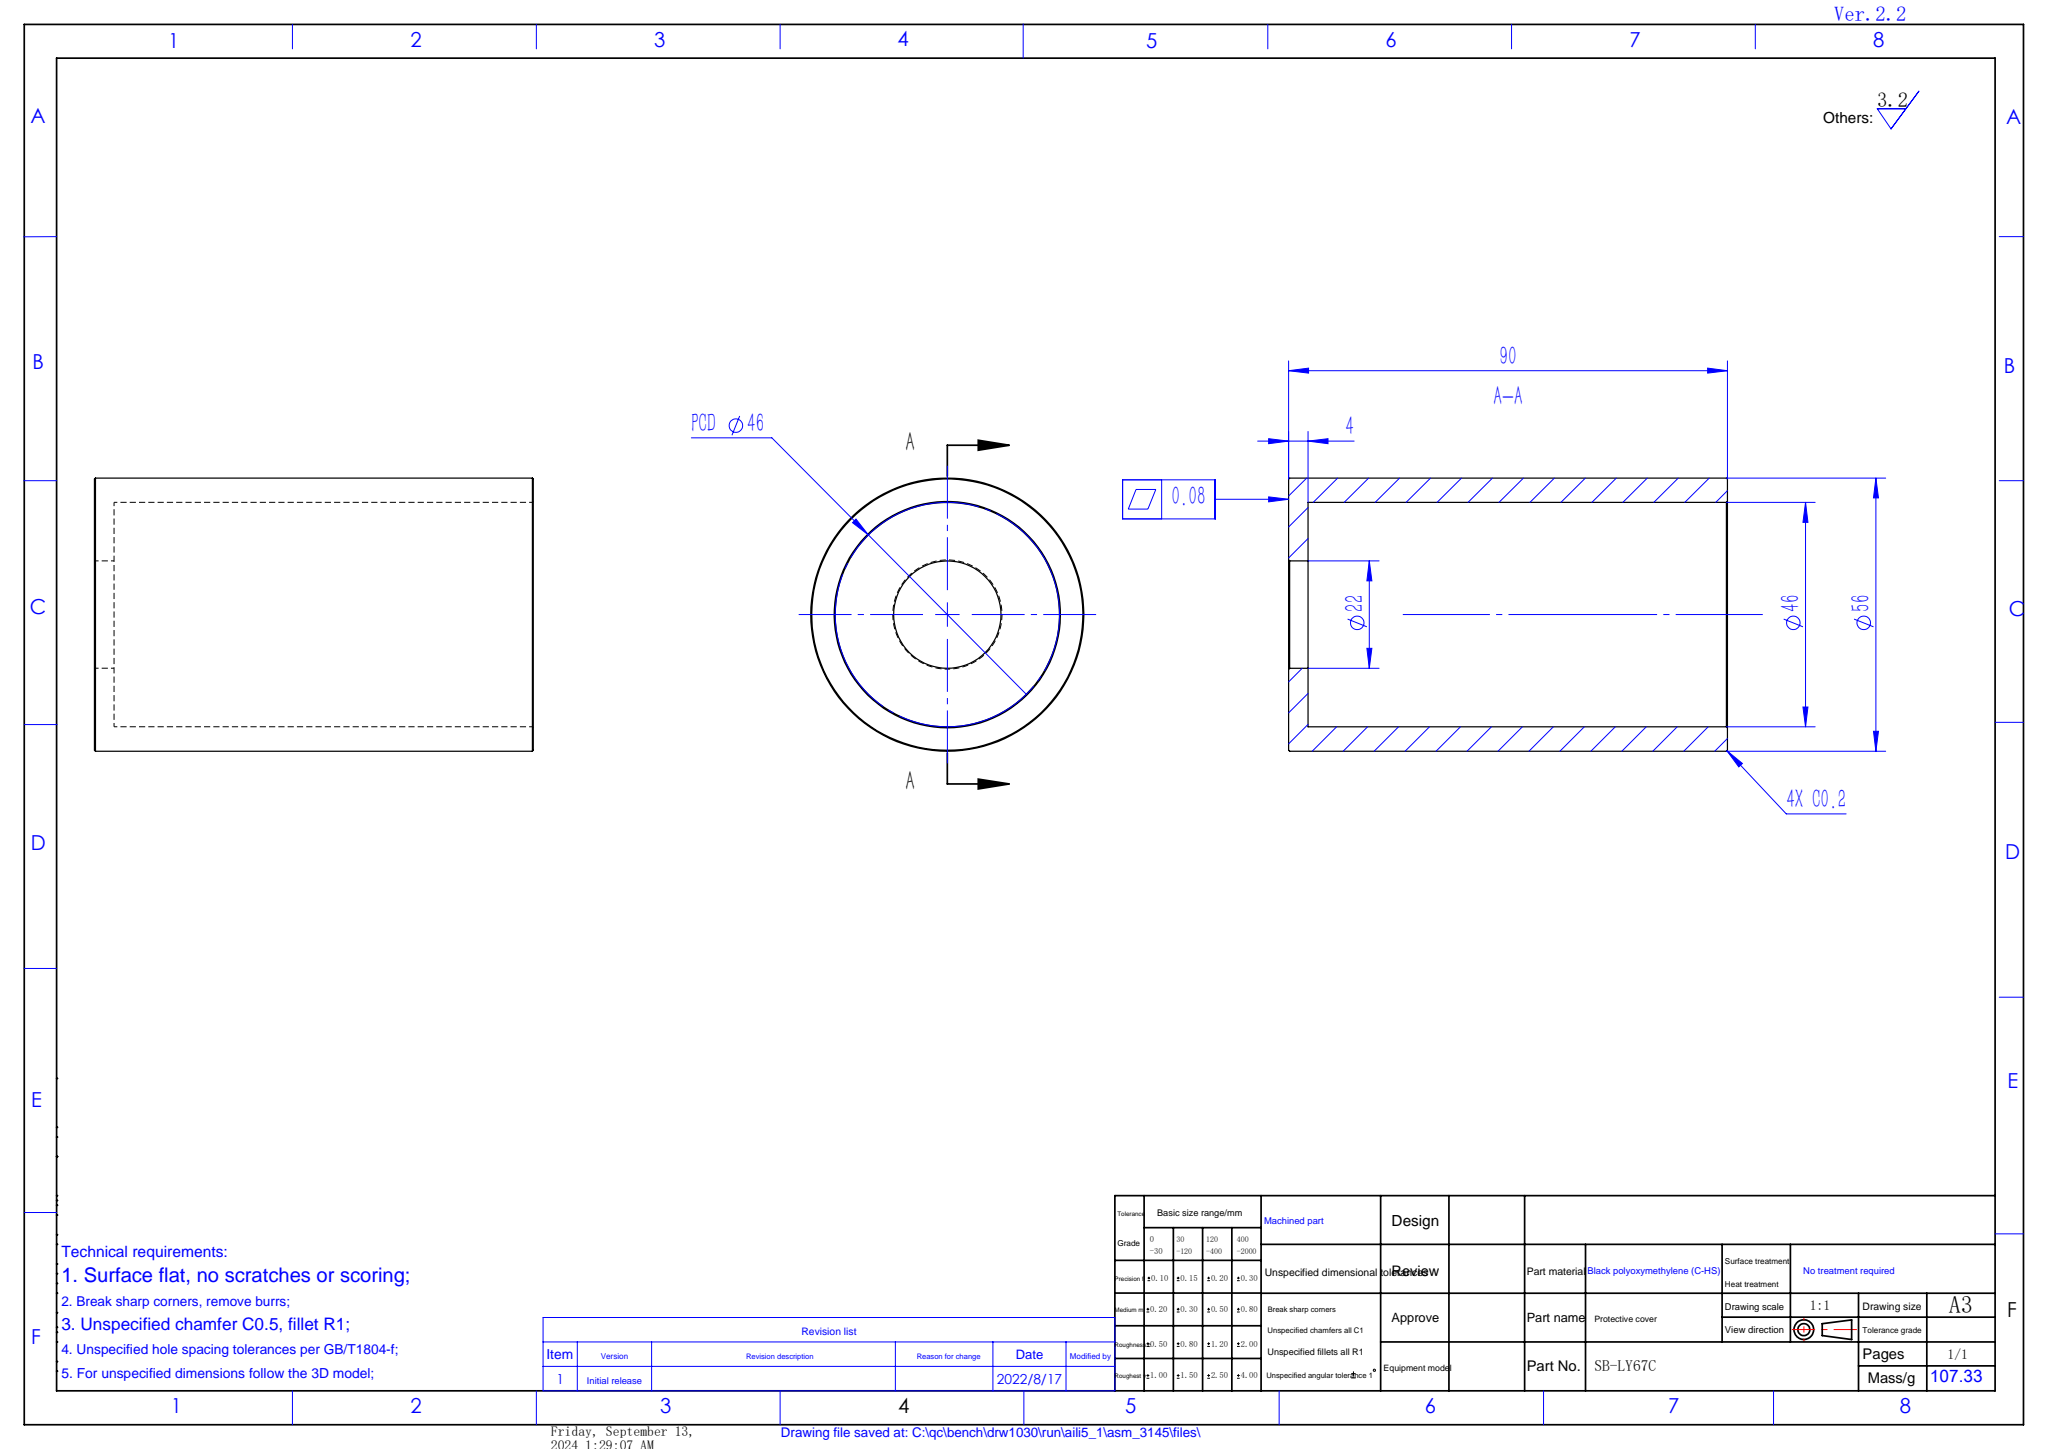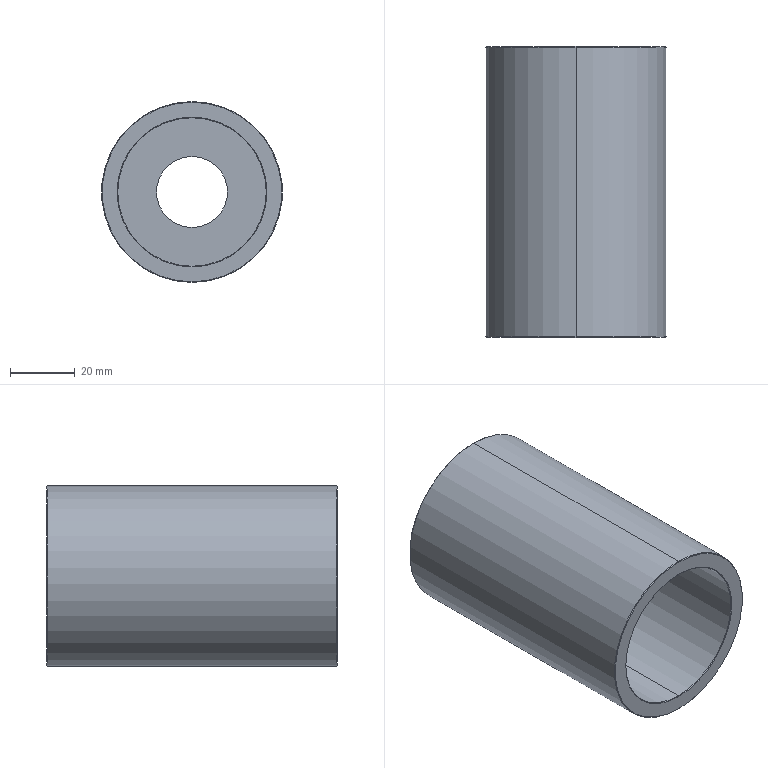Part | SolidWorks | features Chamfer 1, Extrusion 1, ICE 1 | 1 solid | 17 faces | box 56 x 90 x 56 mm | volume 77215 mm3 | cone 8 | cylinder 6 | plane 3 | commonest cylinder face diameters 22 x2 46 x2 56 x2
STEP:
#1=CARTESIAN_POINT('',(0.,0.,-27.8));
#2=VERTEX_POINT('',#1);
#3=CARTESIAN_POINT('',(0.,0.,27.8));
#4=VERTEX_POINT('',#3);
#5=CARTESIAN_POINT('',(0.,0.,0.));
#6=DIRECTION('',(0.,-1.,0.));
#7=DIRECTION('',(0.,0.,1.));
#8=AXIS2_PLACEMENT_3D('',#5,#6,#7);
#9=CIRCLE('',#8,27.8);
#10=EDGE_CURVE('',#2,#4,#9,.T.);
#11=ORIENTED_EDGE('',*,*,#10,.F.);
#12=CARTESIAN_POINT('',(0.,0.2,-28.));
#13=VERTEX_POINT('',#12);
#14=CARTESIAN_POINT('',(0.,0.2,-28.));
#15=DIRECTION('',(0.,0.7071,-0.7071));
#16=VECTOR('',#15,1000.);
#17=LINE('',#14,#16);
#18=EDGE_CURVE('',#2,#13,#17,.T.);
#19=ORIENTED_EDGE('',*,*,#18,.T.);
#20=CARTESIAN_POINT('',(0.,0.2,28.));
#21=VERTEX_POINT('',#20);
#22=CARTESIAN_POINT('',(0.,0.2,0.));
#23=DIRECTION('',(0.,1.,0.));
#24=DIRECTION('',(0.,0.,1.));
#25=AXIS2_PLACEMENT_3D('',#22,#23,#24);
#26=CIRCLE('',#25,28.);
#27=EDGE_CURVE('',#21,#13,#26,.T.);
#28=ORIENTED_EDGE('',*,*,#27,.F.);
#29=CARTESIAN_POINT('',(0.,0.2,28.));
#30=DIRECTION('',(0.,0.7071,0.7071));
#31=VECTOR('',#30,1000.);
#32=LINE('',#29,#31);
#33=EDGE_CURVE('',#4,#21,#32,.T.);
#34=ORIENTED_EDGE('',*,*,#33,.F.);
#35=EDGE_LOOP('',(#11,#19,#28,#34));
#36=FACE_OUTER_BOUND('',#35,.T.);
#37=CARTESIAN_POINT('',(0.,0.2,0.));
#38=DIRECTION('',(0.,1.,0.));
#39=DIRECTION('',(0.,0.,1.));
#40=AXIS2_PLACEMENT_3D('',#37,#38,#39);
#41=CONICAL_SURFACE('',#40,28.,0.7854);
#42=ADVANCED_FACE('',(#36),#41,.T.);
#43=CARTESIAN_POINT('',(0.,90.,27.8));
#44=VERTEX_POINT('',#43);
#45=CARTESIAN_POINT('',(0.,90.,-27.8));
#46=VERTEX_POINT('',#45);
#47=CARTESIAN_POINT('',(0.,90.,0.));
#48=DIRECTION('',(0.,1.,0.));
#49=DIRECTION('',(0.,0.,1.));
#50=AXIS2_PLACEMENT_3D('',#47,#48,#49);
#51=CIRCLE('',#50,27.8);
#52=EDGE_CURVE('',#44,#46,#51,.T.);
#53=ORIENTED_EDGE('',*,*,#52,.F.);
#54=CARTESIAN_POINT('',(0.,89.8,28.));
#55=VERTEX_POINT('',#54);
#56=CARTESIAN_POINT('',(0.,90.,27.8));
#57=DIRECTION('',(0.,-0.7071,0.7071));
#58=VECTOR('',#57,1000.);
#59=LINE('',#56,#58);
#60=EDGE_CURVE('',#44,#55,#59,.T.);
#61=ORIENTED_EDGE('',*,*,#60,.T.);
#62=CARTESIAN_POINT('',(0.,89.8,-28.));
#63=VERTEX_POINT('',#62);
#64=CARTESIAN_POINT('',(0.,89.8,0.));
#65=DIRECTION('',(0.,-1.,0.));
#66=DIRECTION('',(0.,0.,1.));
#67=AXIS2_PLACEMENT_3D('',#64,#65,#66);
#68=CIRCLE('',#67,28.);
#69=EDGE_CURVE('',#63,#55,#68,.T.);
#70=ORIENTED_EDGE('',*,*,#69,.F.);
#71=CARTESIAN_POINT('',(0.,90.,-27.8));
#72=DIRECTION('',(0.,-0.7071,-0.7071));
#73=VECTOR('',#72,1000.);
#74=LINE('',#71,#73);
#75=EDGE_CURVE('',#46,#63,#74,.T.);
#76=ORIENTED_EDGE('',*,*,#75,.F.);
#77=EDGE_LOOP('',(#53,#61,#70,#76));
#78=FACE_OUTER_BOUND('',#77,.T.);
#79=CARTESIAN_POINT('',(0.,90.,0.));
#80=DIRECTION('',(0.,-1.,0.));
#81=DIRECTION('',(0.,0.,-1.));
#82=AXIS2_PLACEMENT_3D('',#79,#80,#81);
#83=CONICAL_SURFACE('',#82,27.8,0.7854);
#84=ADVANCED_FACE('',(#78),#83,.T.);
#85=CARTESIAN_POINT('',(0.,0.2,23.));
#86=VERTEX_POINT('',#85);
#87=CARTESIAN_POINT('',(0.,0.2,-23.));
#88=VERTEX_POINT('',#87);
#89=CARTESIAN_POINT('',(0.,0.2,0.));
#90=DIRECTION('',(0.,-1.,0.));
#91=DIRECTION('',(0.,0.,1.));
#92=AXIS2_PLACEMENT_3D('',#89,#90,#91);
#93=CIRCLE('',#92,23.);
#94=EDGE_CURVE('',#86,#88,#93,.T.);
#95=ORIENTED_EDGE('',*,*,#94,.F.);
#96=CARTESIAN_POINT('',(0.,0.,23.2));
#97=VERTEX_POINT('',#96);
#98=CARTESIAN_POINT('',(0.,0.,23.2));
#99=DIRECTION('',(0.,-0.7071,0.7071));
#100=VECTOR('',#99,1000.);
#101=LINE('',#98,#100);
#102=EDGE_CURVE('',#86,#97,#101,.T.);
#103=ORIENTED_EDGE('',*,*,#102,.T.);
#104=CARTESIAN_POINT('',(0.,0.,-23.2));
#105=VERTEX_POINT('',#104);
#106=CARTESIAN_POINT('',(0.,0.,0.));
#107=DIRECTION('',(0.,1.,0.));
#108=DIRECTION('',(0.,0.,1.));
#109=AXIS2_PLACEMENT_3D('',#106,#107,#108);
#110=CIRCLE('',#109,23.2);
#111=EDGE_CURVE('',#105,#97,#110,.T.);
#112=ORIENTED_EDGE('',*,*,#111,.F.);
#113=CARTESIAN_POINT('',(0.,0.,-23.2));
#114=DIRECTION('',(0.,-0.7071,-0.7071));
#115=VECTOR('',#114,1000.);
#116=LINE('',#113,#115);
#117=EDGE_CURVE('',#88,#105,#116,.T.);
#118=ORIENTED_EDGE('',*,*,#117,.F.);
#119=EDGE_LOOP('',(#95,#103,#112,#118));
#120=FACE_OUTER_BOUND('',#119,.T.);
#121=CARTESIAN_POINT('',(0.,0.,0.));
#122=DIRECTION('',(0.,-1.,0.));
#123=DIRECTION('',(0.,0.,-1.));
#124=AXIS2_PLACEMENT_3D('',#121,#122,#123);
#125=CONICAL_SURFACE('',#124,23.2,0.7854);
#126=ADVANCED_FACE('',(#120),#125,.F.);
#127=CARTESIAN_POINT('',(0.,89.8,-11.));
#128=VERTEX_POINT('',#127);
#129=CARTESIAN_POINT('',(0.,89.8,11.));
#130=VERTEX_POINT('',#129);
#131=CARTESIAN_POINT('',(0.,89.8,0.));
#132=DIRECTION('',(0.,1.,0.));
#133=DIRECTION('',(0.,0.,1.));
#134=AXIS2_PLACEMENT_3D('',#131,#132,#133);
#135=CIRCLE('',#134,11.);
#136=EDGE_CURVE('',#128,#130,#135,.T.);
#137=ORIENTED_EDGE('',*,*,#136,.F.);
#138=CARTESIAN_POINT('',(0.,90.,-11.2));
#139=VERTEX_POINT('',#138);
#140=CARTESIAN_POINT('',(0.,90.,-11.2));
#141=DIRECTION('',(0.,0.7071,-0.7071));
#142=VECTOR('',#141,1000.);
#143=LINE('',#140,#142);
#144=EDGE_CURVE('',#128,#139,#143,.T.);
#145=ORIENTED_EDGE('',*,*,#144,.T.);
#146=CARTESIAN_POINT('',(0.,90.,11.2));
#147=VERTEX_POINT('',#146);
#148=CARTESIAN_POINT('',(0.,90.,0.));
#149=DIRECTION('',(0.,-1.,0.));
#150=DIRECTION('',(0.,0.,1.));
#151=AXIS2_PLACEMENT_3D('',#148,#149,#150);
#152=CIRCLE('',#151,11.2);
#153=EDGE_CURVE('',#147,#139,#152,.T.);
#154=ORIENTED_EDGE('',*,*,#153,.F.);
#155=CARTESIAN_POINT('',(0.,90.,11.2));
#156=DIRECTION('',(0.,0.7071,0.7071));
#157=VECTOR('',#156,1000.);
#158=LINE('',#155,#157);
#159=EDGE_CURVE('',#130,#147,#158,.T.);
#160=ORIENTED_EDGE('',*,*,#159,.F.);
#161=EDGE_LOOP('',(#137,#145,#154,#160));
#162=FACE_OUTER_BOUND('',#161,.T.);
#163=CARTESIAN_POINT('',(0.,90.,0.));
#164=DIRECTION('',(0.,1.,0.));
#165=DIRECTION('',(0.,0.,1.));
#166=AXIS2_PLACEMENT_3D('',#163,#164,#165);
#167=CONICAL_SURFACE('',#166,11.2,0.7854);
#168=ADVANCED_FACE('',(#162),#167,.F.);
#169=CARTESIAN_POINT('',(0.,86.,11.));
#170=VERTEX_POINT('',#169);
#171=CARTESIAN_POINT('',(0.,86.,-11.));
#172=VERTEX_POINT('',#171);
#173=CARTESIAN_POINT('',(0.,86.,0.));
#174=DIRECTION('',(0.,-1.,0.));
#175=DIRECTION('',(0.,0.,-1.));
#176=AXIS2_PLACEMENT_3D('',#173,#174,#175);
#177=CIRCLE('',#176,11.);
#178=EDGE_CURVE('',#170,#172,#177,.T.);
#179=ORIENTED_EDGE('',*,*,#178,.T.);
#180=CARTESIAN_POINT('',(0.,86.,-11.));
#181=DIRECTION('',(0.,1.,0.));
#182=VECTOR('',#181,1000.);
#183=LINE('',#180,#182);
#184=EDGE_CURVE('',#172,#128,#183,.T.);
#185=ORIENTED_EDGE('',*,*,#184,.T.);
#186=ORIENTED_EDGE('',*,*,#136,.T.);
#187=CARTESIAN_POINT('',(0.,86.,11.));
#188=DIRECTION('',(0.,1.,0.));
#189=VECTOR('',#188,1000.);
#190=LINE('',#187,#189);
#191=EDGE_CURVE('',#170,#130,#190,.T.);
#192=ORIENTED_EDGE('',*,*,#191,.F.);
#193=EDGE_LOOP('',(#179,#185,#186,#192));
#194=FACE_OUTER_BOUND('',#193,.T.);
#195=CARTESIAN_POINT('',(0.,86.,0.));
#196=DIRECTION('',(0.,1.,0.));
#197=DIRECTION('',(0.,0.,1.));
#198=AXIS2_PLACEMENT_3D('',#195,#196,#197);
#199=CYLINDRICAL_SURFACE('',#198,11.);
#200=ADVANCED_FACE('',(#194),#199,.F.);
#201=CARTESIAN_POINT('',(0.,86.,23.));
#202=VERTEX_POINT('',#201);
#203=CARTESIAN_POINT('',(0.,86.,-23.));
#204=VERTEX_POINT('',#203);
#205=CARTESIAN_POINT('',(0.,86.,0.));
#206=DIRECTION('',(0.,-1.,0.));
#207=DIRECTION('',(0.,0.,-1.));
#208=AXIS2_PLACEMENT_3D('',#205,#206,#207);
#209=CIRCLE('',#208,23.);
#210=EDGE_CURVE('',#202,#204,#209,.T.);
#211=ORIENTED_EDGE('',*,*,#210,.F.);
#212=CARTESIAN_POINT('',(0.,90.,23.));
#213=DIRECTION('',(0.,-1.,0.));
#214=VECTOR('',#213,1000.);
#215=LINE('',#212,#214);
#216=EDGE_CURVE('',#202,#86,#215,.T.);
#217=ORIENTED_EDGE('',*,*,#216,.T.);
#218=ORIENTED_EDGE('',*,*,#94,.T.);
#219=CARTESIAN_POINT('',(0.,90.,-23.));
#220=DIRECTION('',(0.,-1.,0.));
#221=VECTOR('',#220,1000.);
#222=LINE('',#219,#221);
#223=EDGE_CURVE('',#204,#88,#222,.T.);
#224=ORIENTED_EDGE('',*,*,#223,.F.);
#225=EDGE_LOOP('',(#211,#217,#218,#224));
#226=FACE_OUTER_BOUND('',#225,.T.);
#227=CARTESIAN_POINT('',(0.,90.,0.));
#228=DIRECTION('',(0.,-1.,0.));
#229=DIRECTION('',(0.,0.,-1.));
#230=AXIS2_PLACEMENT_3D('',#227,#228,#229);
#231=CYLINDRICAL_SURFACE('',#230,23.);
#232=ADVANCED_FACE('',(#226),#231,.F.);
#233=ORIENTED_EDGE('',*,*,#69,.T.);
#234=CARTESIAN_POINT('',(0.,90.,28.));
#235=DIRECTION('',(0.,-1.,0.));
#236=VECTOR('',#235,1000.);
#237=LINE('',#234,#236);
#238=EDGE_CURVE('',#55,#21,#237,.T.);
#239=ORIENTED_EDGE('',*,*,#238,.T.);
#240=ORIENTED_EDGE('',*,*,#27,.T.);
#241=CARTESIAN_POINT('',(0.,90.,-28.));
#242=DIRECTION('',(0.,-1.,0.));
#243=VECTOR('',#242,1000.);
#244=LINE('',#241,#243);
#245=EDGE_CURVE('',#63,#13,#244,.T.);
#246=ORIENTED_EDGE('',*,*,#245,.F.);
#247=EDGE_LOOP('',(#233,#239,#240,#246));
#248=FACE_OUTER_BOUND('',#247,.T.);
#249=CARTESIAN_POINT('',(0.,90.,0.));
#250=DIRECTION('',(0.,-1.,0.));
#251=DIRECTION('',(0.,0.,-1.));
#252=AXIS2_PLACEMENT_3D('',#249,#250,#251);
#253=CYLINDRICAL_SURFACE('',#252,28.);
#254=ADVANCED_FACE('',(#248),#253,.T.);
#255=ORIENTED_EDGE('',*,*,#153,.T.);
#256=CARTESIAN_POINT('',(0.,90.,0.));
#257=DIRECTION('',(0.,-1.,0.));
#258=DIRECTION('',(0.,0.,1.));
#259=AXIS2_PLACEMENT_3D('',#256,#257,#258);
#260=CIRCLE('',#259,11.2);
#261=EDGE_CURVE('',#139,#147,#260,.T.);
#262=ORIENTED_EDGE('',*,*,#261,.T.);
#263=EDGE_LOOP('',(#255,#262));
#264=FACE_BOUND('',#263,.T.);
#265=CARTESIAN_POINT('',(0.,90.,0.));
#266=DIRECTION('',(0.,1.,0.));
#267=DIRECTION('',(0.,0.,1.));
#268=AXIS2_PLACEMENT_3D('',#265,#266,#267);
#269=CIRCLE('',#268,27.8);
#270=EDGE_CURVE('',#46,#44,#269,.T.);
#271=ORIENTED_EDGE('',*,*,#270,.T.);
#272=ORIENTED_EDGE('',*,*,#52,.T.);
#273=EDGE_LOOP('',(#271,#272));
#274=FACE_OUTER_BOUND('',#273,.T.);
#275=CARTESIAN_POINT('',(0.,90.,0.));
#276=DIRECTION('',(0.,1.,0.));
#277=DIRECTION('',(0.,0.,1.));
#278=AXIS2_PLACEMENT_3D('',#275,#276,#277);
#279=PLANE('',#278);
#280=ADVANCED_FACE('',(#264,#274),#279,.T.);
#281=ORIENTED_EDGE('',*,*,#111,.T.);
#282=CARTESIAN_POINT('',(0.,0.,0.));
#283=DIRECTION('',(0.,1.,0.));
#284=DIRECTION('',(0.,0.,1.));
#285=AXIS2_PLACEMENT_3D('',#282,#283,#284);
#286=CIRCLE('',#285,23.2);
#287=EDGE_CURVE('',#97,#105,#286,.T.);
#288=ORIENTED_EDGE('',*,*,#287,.T.);
#289=EDGE_LOOP('',(#281,#288));
#290=FACE_BOUND('',#289,.T.);
#291=CARTESIAN_POINT('',(0.,0.,0.));
#292=DIRECTION('',(0.,-1.,0.));
#293=DIRECTION('',(0.,0.,1.));
#294=AXIS2_PLACEMENT_3D('',#291,#292,#293);
#295=CIRCLE('',#294,27.8);
#296=EDGE_CURVE('',#4,#2,#295,.T.);
#297=ORIENTED_EDGE('',*,*,#296,.T.);
#298=ORIENTED_EDGE('',*,*,#10,.T.);
#299=EDGE_LOOP('',(#297,#298));
#300=FACE_OUTER_BOUND('',#299,.T.);
#301=CARTESIAN_POINT('',(0.,0.,0.));
#302=DIRECTION('',(0.,1.,0.));
#303=DIRECTION('',(0.,0.,1.));
#304=AXIS2_PLACEMENT_3D('',#301,#302,#303);
#305=PLANE('',#304);
#306=ADVANCED_FACE('',(#290,#300),#305,.F.);
#307=ORIENTED_EDGE('',*,*,#238,.F.);
#308=CARTESIAN_POINT('',(0.,89.8,0.));
#309=DIRECTION('',(0.,-1.,0.));
#310=DIRECTION('',(0.,0.,1.));
#311=AXIS2_PLACEMENT_3D('',#308,#309,#310);
#312=CIRCLE('',#311,28.);
#313=EDGE_CURVE('',#55,#63,#312,.T.);
#314=ORIENTED_EDGE('',*,*,#313,.T.);
#315=ORIENTED_EDGE('',*,*,#245,.T.);
#316=CARTESIAN_POINT('',(0.,0.2,0.));
#317=DIRECTION('',(0.,1.,0.));
#318=DIRECTION('',(0.,0.,1.));
#319=AXIS2_PLACEMENT_3D('',#316,#317,#318);
#320=CIRCLE('',#319,28.);
#321=EDGE_CURVE('',#13,#21,#320,.T.);
#322=ORIENTED_EDGE('',*,*,#321,.T.);
#323=EDGE_LOOP('',(#307,#314,#315,#322));
#324=FACE_OUTER_BOUND('',#323,.T.);
#325=CARTESIAN_POINT('',(0.,90.,0.));
#326=DIRECTION('',(0.,-1.,0.));
#327=DIRECTION('',(0.,0.,-1.));
#328=AXIS2_PLACEMENT_3D('',#325,#326,#327);
#329=CYLINDRICAL_SURFACE('',#328,28.);
#330=ADVANCED_FACE('',(#324),#329,.T.);
#331=ORIENTED_EDGE('',*,*,#216,.F.);
#332=CARTESIAN_POINT('',(0.,86.,0.));
#333=DIRECTION('',(0.,-1.,0.));
#334=DIRECTION('',(0.,0.,-1.));
#335=AXIS2_PLACEMENT_3D('',#332,#333,#334);
#336=CIRCLE('',#335,23.);
#337=EDGE_CURVE('',#204,#202,#336,.T.);
#338=ORIENTED_EDGE('',*,*,#337,.F.);
#339=ORIENTED_EDGE('',*,*,#223,.T.);
#340=CARTESIAN_POINT('',(0.,0.2,0.));
#341=DIRECTION('',(0.,-1.,0.));
#342=DIRECTION('',(0.,0.,1.));
#343=AXIS2_PLACEMENT_3D('',#340,#341,#342);
#344=CIRCLE('',#343,23.);
#345=EDGE_CURVE('',#88,#86,#344,.T.);
#346=ORIENTED_EDGE('',*,*,#345,.T.);
#347=EDGE_LOOP('',(#331,#338,#339,#346));
#348=FACE_OUTER_BOUND('',#347,.T.);
#349=CARTESIAN_POINT('',(0.,90.,0.));
#350=DIRECTION('',(0.,-1.,0.));
#351=DIRECTION('',(0.,0.,-1.));
#352=AXIS2_PLACEMENT_3D('',#349,#350,#351);
#353=CYLINDRICAL_SURFACE('',#352,23.);
#354=ADVANCED_FACE('',(#348),#353,.F.);
#355=ORIENTED_EDGE('',*,*,#178,.F.);
#356=CARTESIAN_POINT('',(0.,86.,0.));
#357=DIRECTION('',(0.,-1.,0.));
#358=DIRECTION('',(0.,0.,-1.));
#359=AXIS2_PLACEMENT_3D('',#356,#357,#358);
#360=CIRCLE('',#359,11.);
#361=EDGE_CURVE('',#172,#170,#360,.T.);
#362=ORIENTED_EDGE('',*,*,#361,.F.);
#363=EDGE_LOOP('',(#355,#362));
#364=FACE_BOUND('',#363,.T.);
#365=ORIENTED_EDGE('',*,*,#337,.T.);
#366=ORIENTED_EDGE('',*,*,#210,.T.);
#367=EDGE_LOOP('',(#365,#366));
#368=FACE_OUTER_BOUND('',#367,.T.);
#369=CARTESIAN_POINT('',(0.,86.,0.));
#370=DIRECTION('',(0.,-1.,0.));
#371=DIRECTION('',(0.,0.,-1.));
#372=AXIS2_PLACEMENT_3D('',#369,#370,#371);
#373=PLANE('',#372);
#374=ADVANCED_FACE('',(#364,#368),#373,.T.);
#375=ORIENTED_EDGE('',*,*,#184,.F.);
#376=ORIENTED_EDGE('',*,*,#361,.T.);
#377=ORIENTED_EDGE('',*,*,#191,.T.);
#378=CARTESIAN_POINT('',(0.,89.8,0.));
#379=DIRECTION('',(0.,1.,0.));
#380=DIRECTION('',(0.,0.,1.));
#381=AXIS2_PLACEMENT_3D('',#378,#379,#380);
#382=CIRCLE('',#381,11.);
#383=EDGE_CURVE('',#130,#128,#382,.T.);
#384=ORIENTED_EDGE('',*,*,#383,.T.);
#385=EDGE_LOOP('',(#375,#376,#377,#384));
#386=FACE_OUTER_BOUND('',#385,.T.);
#387=CARTESIAN_POINT('',(0.,86.,0.));
#388=DIRECTION('',(0.,1.,0.));
#389=DIRECTION('',(0.,0.,1.));
#390=AXIS2_PLACEMENT_3D('',#387,#388,#389);
#391=CYLINDRICAL_SURFACE('',#390,11.);
#392=ADVANCED_FACE('',(#386),#391,.F.);
#393=ORIENTED_EDGE('',*,*,#144,.F.);
#394=ORIENTED_EDGE('',*,*,#383,.F.);
#395=ORIENTED_EDGE('',*,*,#159,.T.);
#396=ORIENTED_EDGE('',*,*,#261,.F.);
#397=EDGE_LOOP('',(#393,#394,#395,#396));
#398=FACE_OUTER_BOUND('',#397,.T.);
#399=CARTESIAN_POINT('',(0.,90.,0.));
#400=DIRECTION('',(0.,1.,0.));
#401=DIRECTION('',(0.,0.,1.));
#402=AXIS2_PLACEMENT_3D('',#399,#400,#401);
#403=CONICAL_SURFACE('',#402,11.2,0.7854);
#404=ADVANCED_FACE('',(#398),#403,.F.);
#405=ORIENTED_EDGE('',*,*,#102,.F.);
#406=ORIENTED_EDGE('',*,*,#345,.F.);
#407=ORIENTED_EDGE('',*,*,#117,.T.);
#408=ORIENTED_EDGE('',*,*,#287,.F.);
#409=EDGE_LOOP('',(#405,#406,#407,#408));
#410=FACE_OUTER_BOUND('',#409,.T.);
#411=CARTESIAN_POINT('',(0.,0.,0.));
#412=DIRECTION('',(0.,-1.,0.));
#413=DIRECTION('',(0.,0.,-1.));
#414=AXIS2_PLACEMENT_3D('',#411,#412,#413);
#415=CONICAL_SURFACE('',#414,23.2,0.7854);
#416=ADVANCED_FACE('',(#410),#415,.F.);
#417=ORIENTED_EDGE('',*,*,#60,.F.);
#418=ORIENTED_EDGE('',*,*,#270,.F.);
#419=ORIENTED_EDGE('',*,*,#75,.T.);
#420=ORIENTED_EDGE('',*,*,#313,.F.);
#421=EDGE_LOOP('',(#417,#418,#419,#420));
#422=FACE_OUTER_BOUND('',#421,.T.);
#423=CARTESIAN_POINT('',(0.,90.,0.));
#424=DIRECTION('',(0.,-1.,0.));
#425=DIRECTION('',(0.,0.,-1.));
#426=AXIS2_PLACEMENT_3D('',#423,#424,#425);
#427=CONICAL_SURFACE('',#426,27.8,0.7854);
#428=ADVANCED_FACE('',(#422),#427,.T.);
#429=ORIENTED_EDGE('',*,*,#18,.F.);
#430=ORIENTED_EDGE('',*,*,#296,.F.);
#431=ORIENTED_EDGE('',*,*,#33,.T.);
#432=ORIENTED_EDGE('',*,*,#321,.F.);
#433=EDGE_LOOP('',(#429,#430,#431,#432));
#434=FACE_OUTER_BOUND('',#433,.T.);
#435=CARTESIAN_POINT('',(0.,0.2,0.));
#436=DIRECTION('',(0.,1.,0.));
#437=DIRECTION('',(0.,0.,1.));
#438=AXIS2_PLACEMENT_3D('',#435,#436,#437);
#439=CONICAL_SURFACE('',#438,28.,0.7854);
#440=ADVANCED_FACE('',(#434),#439,.T.);
#441=CLOSED_SHELL('',(#42,#84,#126,#168,#200,#232,#254,#280,#306,#330,#354,#374,#392,#404,#416,#428,#440));
#442=MANIFOLD_SOLID_BREP('',#441);
#443=CARTESIAN_POINT('',(0.,0.,0.));
#444=DIRECTION('',(0.,0.,1.));
#445=DIRECTION('',(1.,0.,0.));
#446=AXIS2_PLACEMENT_3D('',#443,#444,#445);
#447=(LENGTH_UNIT()NAMED_UNIT(*)SI_UNIT(.MILLI.,.METRE.));
#448=UNCERTAINTY_MEASURE_WITH_UNIT(LENGTH_MEASURE(0.00001),#447,'','');
#449=(NAMED_UNIT(*)PLANE_ANGLE_UNIT()SI_UNIT($,.RADIAN.));
#450=(NAMED_UNIT(*)SI_UNIT($,.STERADIAN.)SOLID_ANGLE_UNIT());
#451=(GEOMETRIC_REPRESENTATION_CONTEXT(3)GLOBAL_UNCERTAINTY_ASSIGNED_CONTEXT((#448))GLOBAL_UNIT_ASSIGNED_CONTEXT((#447,#449,#450))REPRESENTATION_CONTEXT('',''));
#452=ADVANCED_BREP_SHAPE_REPRESENTATION('',(#442,#446),#451);